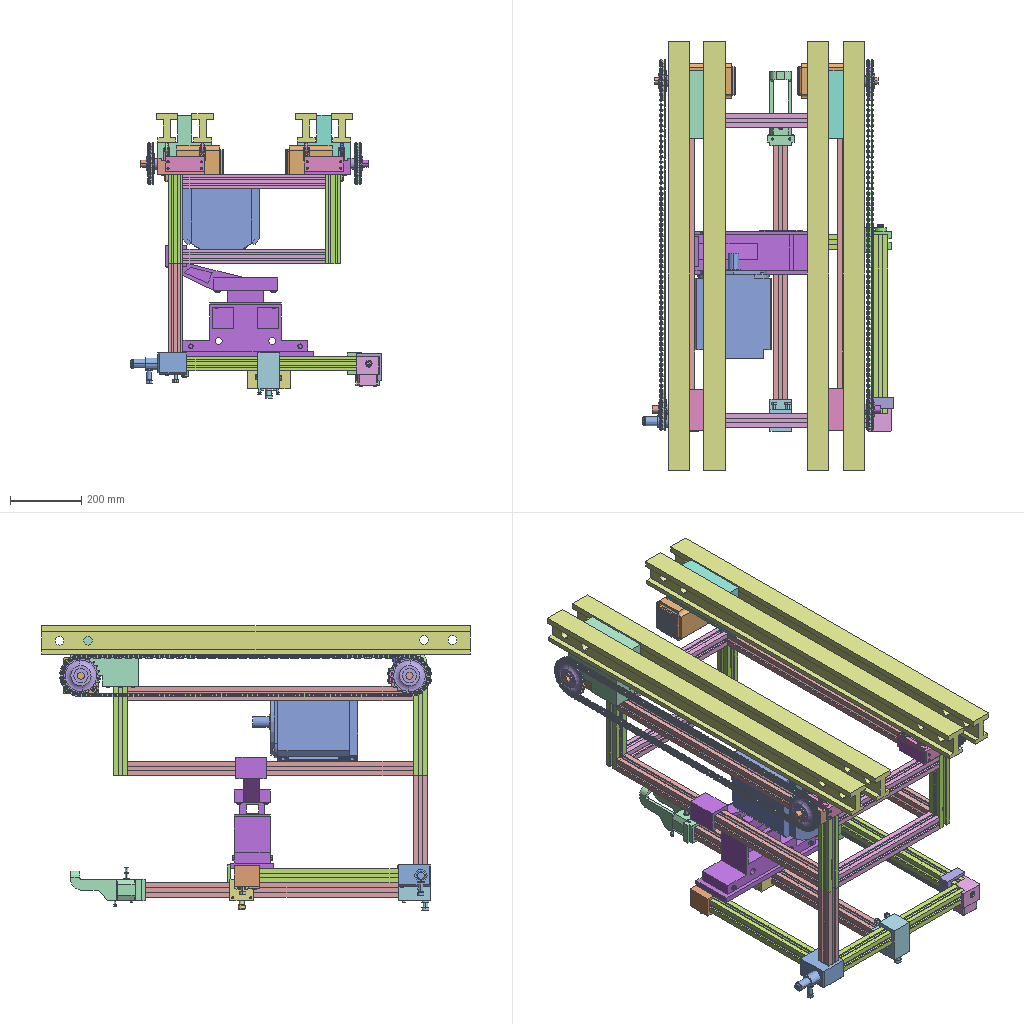Assembly | SolidWorks | 26 different items | 405 placed | box 701 x 1200 x 797 mm
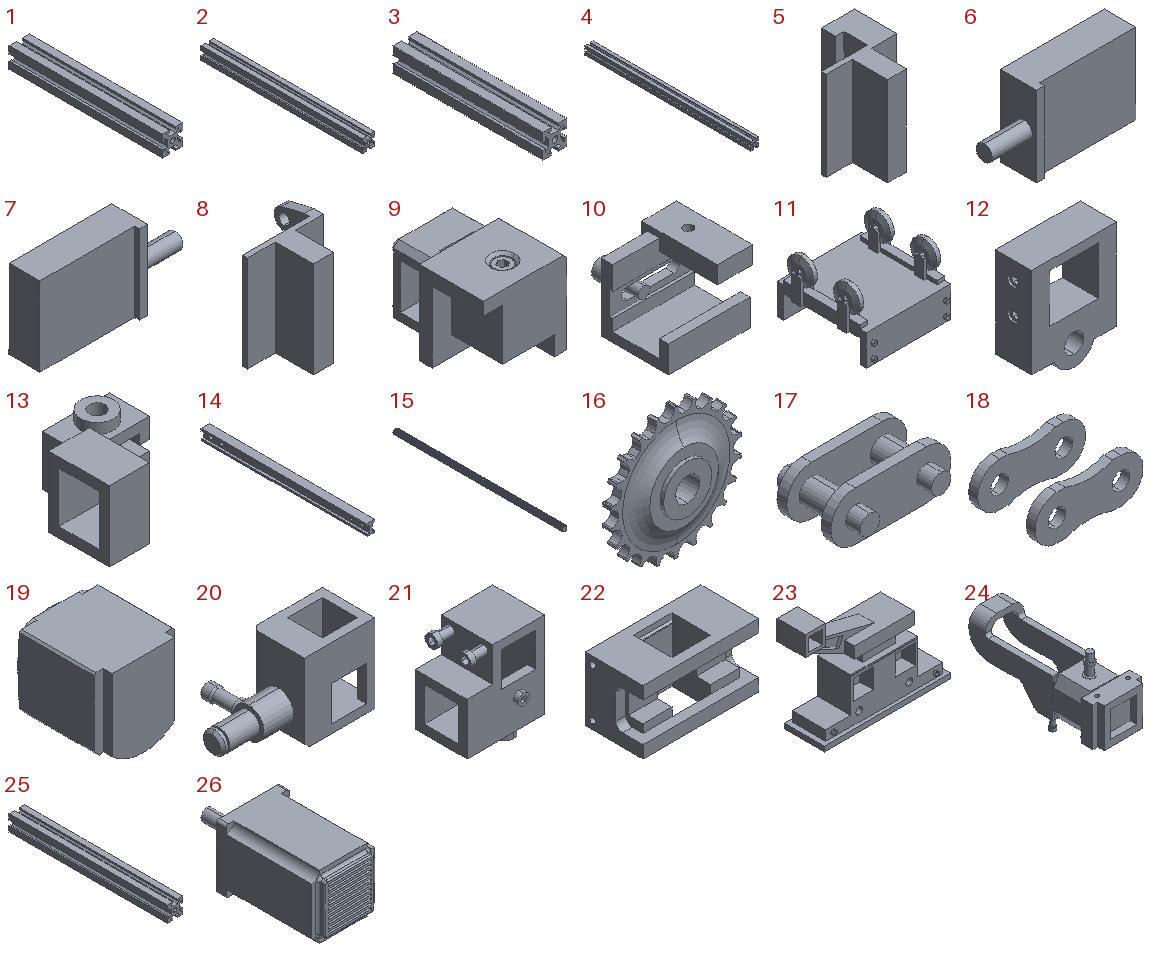Parts list (item | quantity | size | volume | features):
1 | x1 | 40 x 300 x 40 mm | 272732 mm3 | features Extrusion 1
2 | x4 | 40 x 500 x 40 mm | 454553 mm3 | features Extrusion 1
3 | x4 | 40 x 250 x 40 mm | 227277 mm3 | features Extrusion 1
4 | x5 | 40 x 800 x 40 mm | 727286 mm3 | features Extrusion 1
5 | x1 | 150 x 169 x 189.781 mm | 1407885 mm3 | features ICE 7, Extrusion 1, MirrorSolid 1
6 | x1 | 180 x 49 x 100 mm | 529109 mm3 | features ICE 6, Extrusion 1, MirrorSolid 1
7 | x1 | 180 x 49 x 100 mm | 529109 mm3 | features ICE 5, Extrusion 1
8 | x1 | 150 x 169 x 189.781 mm | 1407885 mm3 | features ICE 6, Extrusion 1
9 | x1 | 65 x 84 x 65 mm | 191550 mm3 | features ICE 10, Chamfer 3, Extrusion 1
10 | x1 | 70 x 83 x 63 mm | 98989 mm3 | features ICE 11, Extrusion 1
11 | x2 | 117 x 123 x 81 mm | 229130 mm3 | features ICE 7, LPattern 4, Chamfer 1, Extrusion 1, MirrorPattern 1, Revolution 1
12 | x1 | 70 x 30 x 86.838 mm | 111034 mm3 | features ICE 5, Extrusion 1, MirrorPattern 1
13 | x1 | 90 x 90 x 70 mm | 165265 mm3 | features ICE 5, Extrusion 1
14 | x4 | 60 x 1200 x 80 mm | 3164730 mm3 | features Extrusion 1, ICE 1
15 | x1 | 17 x 560 x 17 mm | 93030 mm3 | features Extrusion 1, Helix 1, ICE 1, Sweep 1
16 | x4 | 108.11 x 33 x 108.911 mm | 101426 mm3 | features ICE 2, Extrusion 1, RefAxis 1, RevCut 1
17 | x180 | 24.52 x 17 x 10 mm | 1321 mm3 | features ICE 4, RefPoint 2, Extrusion 1
18 | x180 | 24.52 x 15 x 10 mm | 736.592 mm3 | features ICE 2, Extrusion 1
19 | x1 | 215.394 x 294 x 225 mm | 10267409 mm3 | features ICE 13, Chamfer 1, CirPattern 1, Extrusion 1, MirrorPattern 1
20 | x1 | 156 x 86.375 x 90 mm | 325727 mm3 | features ICE 13, Chamfer 4, Extrusion 1
21 | x1 | 90 x 72 x 127 mm | 255195 mm3 | features ICE 12, Extrusion 1
22 | x1 | 120 x 84 x 66 mm | 274299 mm3 | features ICE 12, Chamfer 2, Fillet 2, Extrusion 1
23 | x1 | 415 x 120 x 311.384 mm | 4368887 mm3 | features ICE 14, MirrorPattern 9, Extrusion 1
24 | x1 | 75 x 208.792 x 108 mm | 304724 mm3 | features ICE 21, Fillet 6, MirrorPattern 3, Chamfer 2, Extrusion 1
25 | x4 | 40 x 400 x 40 mm | 363643 mm3 | features Extrusion 1
26 | x2 | 100 x 225 x 100 mm | 1510650 mm3 | features ICE 6, Fillet 3, CirPattern 1, Extrusion 1, LPattern 1
Mates (type | each side: item.copy, entity, surface, feature):
Coincident | 4.1 face plane Boss-Extrude1 | 3.1 face plane Boss-Extrude1 | 3 times
Coincident | 4.2 face plane Boss-Extrude1 | 3.2 face plane Boss-Extrude1 | 3 times
Coincident | 3.1 face plane Boss-Extrude1 | 25.1 face plane Boss-Extrude1 | 3 times
Coincident | 3.2 face plane Boss-Extrude1 | 25.1 face plane Boss-Extrude1 | 3 times
Coincident | 3.1 face plane Boss-Extrude1 | 25.2 face plane Boss-Extrude1
Coincident | 3.2 face plane Boss-Extrude1 | 25.2 face plane Boss-Extrude1 | 2 times
Coincident | 4.2 face plane Boss-Extrude1 | 3.3 face plane Boss-Extrude1 | 3 times
Coincident | 4.1 face plane Boss-Extrude1 | 3.4 face plane Boss-Extrude1 | 3 times
Coincident | 3.3 face plane Boss-Extrude1 | 25.3 face plane Boss-Extrude1 | 2 times
Coincident | 3.4 face plane Boss-Extrude1 | 25.3 face plane Boss-Extrude1
Coincident | 3.3 face plane Boss-Extrude1 | 25.4 face plane Boss-Extrude1 | 3 times
Coincident | 3.2 face plane Boss-Extrude1 | 4.3 face plane Boss-Extrude1 | 3 times
Coincident | 3.4 face plane Boss-Extrude1 | 4.4 face plane Boss-Extrude1 | 3 times
Coincident | 19.1 face plane Boss-Extrude2 | 4.4 face plane Boss-Extrude1
Coincident | 19.1 face plane Boss-Extrude5 | 4.4 face plane Boss-Extrude1
Concentric | 8.1 face cylinder Boss-Extrude4 | 26.1 face cylinder Boss-Extrude1
Coincident | 8.1 face plane Boss-Extrude4 | 26.1 face plane Boss-Extrude2
Concentric | 26.1 face cylinder Boss-Extrude1 | 16.1 face cylinder Boss-Extrude1
Coincident | 8.1 face plane Boss-Extrude1 | 16.1 face plane Boss-Extrude4
Coincident | 8.1 face plane Boss-Extrude7 | 14.1 face plane Boss-Extrude1
Coincident | 8.1 face plane Boss-Extrude6 | 14.1 face plane Boss-Extrude1
DistanceDim | 8.1 face plane Boss-Extrude5 | 14.1 face plane Boss-Extrude1
Coincident | 4.3 face plane Boss-Extrude1 | 7.1 face plane Boss-Extrude1
Coincident | 3.3 face plane Boss-Extrude1 | 7.1 face plane Boss-Extrude1
Concentric | 7.1 face cylinder Boss-Extrude3 | 16.2 face cylinder Boss-Extrude1
Coincident | 4.3 face plane Boss-Extrude1 | 8.1 face plane Boss-Extrude1 | 2 times
Coincident | 7.1 face plane Boss-Extrude1 | 16.2 face plane Boss-Extrude4
BeltDim | 16.1 face cylinder Cut-Revolve1 | 16.2 face cylinder Cut-Revolve1
Coincident | 8.1 face plane Boss-Extrude6 | 14.2 face plane Boss-Extrude1
Coincident | 8.1 face plane Boss-Extrude7 | 14.2 face plane Boss-Extrude1
Coincident | 14.1 face plane Boss-Extrude1 | 14.2 face plane Boss-Extrude1
DistanceDim | 25.2 face plane Boss-Extrude1 | 8.1 face plane Boss-Extrude1
Concentric | 26.2 face cylinder Boss-Extrude1 | 5.1 face cylinder Mirror3
Coincident | 14.3 face plane Boss-Extrude1 | 5.1 face plane Boss-Extrude7
Coincident | 4.4 face plane Boss-Extrude1 | 5.1 face plane Mirror3
Coincident | 3.4 face plane Boss-Extrude1 | 6.1 face plane Boss-Extrude1
Coincident | 4.4 face plane Boss-Extrude1 | 6.1 face plane Boss-Extrude1
Concentric | 6.1 face cylinder Mirror1 | 16.3 face cylinder Boss-Extrude1
Coincident | 6.1 face plane Mirror1 | 16.3 face plane Boss-Extrude4
Concentric | 26.2 face cylinder Boss-Extrude1 | 16.4 face cylinder Boss-Extrude1
Coincident | 5.1 face plane Boss-Extrude1 | 16.4 face plane Boss-Extrude4
Tangent | 14.1 face plane Boss-Extrude1 | 11.1 face cylinder LPattern4
DistanceDim | 11.1 face plane LPattern4 | 14.1 face plane Boss-Extrude1
Coincident | 7.1 face plane Boss-Extrude1 | 11.1 face plane Boss-Extrude1
Coincident | 8.1 face plane Boss-Extrude6 | 26.1 face plane Boss-Extrude3
Coincident | 3.4 face plane Boss-Extrude1 | 1.1 face plane Boss-Extrude1 | 3 times
Coincident | 1.1 face plane Boss-Extrude1 | 20.1 face plane Cut-Extrude1 | 3 times
Coincident | 1.1 face plane Boss-Extrude1 | 2.1 face plane Boss-Extrude1
Coincident | 20.1 face plane Cut-Extrude3 | 2.1 face plane Boss-Extrude1
Coincident | 20.1 face plane Cut-Extrude1 | 2.1 face plane Boss-Extrude1
Coincident | 20.1 face plane Cut-Extrude1 | 2.2 face plane Boss-Extrude1 | 2 times
Coincident | 1.1 face plane Boss-Extrude1 | 2.2 face plane Boss-Extrude1
Coincident | 2.2 face plane Boss-Extrude1 | 2.3 face plane Boss-Extrude1 | 3 times
Coincident | 2.3 face plane Boss-Extrude1 | 2.4 face plane Boss-Extrude1 | 2 times
Coincident | 2.3 face plane Boss-Extrude1 | 9.1 face plane Boss-Extrude1
Coincident | 2.2 face plane Boss-Extrude1 | 9.1 face plane Boss-Extrude1
Coincident | 2.2 face plane Boss-Extrude1 | 9.1 face plane Boss-Extrude3
Coincident | 2.1 face plane Boss-Extrude1 | 2.4 face plane Boss-Extrude1
Coincident | 2.1 face plane Boss-Extrude1 | 10.1 face plane Boss-Extrude1 | 2 times
Coincident | 2.3 face plane Boss-Extrude1 | 12.1 face plane Boss-Extrude1 | 2 times
Coincident | 9.1 face plane Boss-Extrude1 | 12.1 face plane Boss-Extrude1
Coincident | 2.1 face plane Boss-Extrude1 | 10.1 face plane Boss-Extrude8
Coincident | 2.4 face plane Boss-Extrude1 | 13.1 face plane Boss-Extrude3 | 2 times
Coincident | 2.3 face plane Boss-Extrude1 | 13.1 face plane Boss-Extrude3
Concentric | 13.1 face cylinder Cut-Extrude1 | 15.1 face cylinder Boss-Extrude1
DistanceDim | 13.1 face plane Boss-Extrude5 | 15.1 face plane Cut-Extrude1
Coincident | 2.2 face plane Boss-Extrude1 | 21.1 face plane Boss-Extrude1
Coincident | 2.2 face plane Boss-Extrude1 | 21.1 face plane Cut-Extrude2
DistanceDim | 21.1 face plane Boss-Extrude1 | 9.1 face plane Boss-Extrude1
Coincident | 21.1 face plane Cut-Extrude1 | 4.5 face plane Boss-Extrude1 | 2 times
Coincident | 21.1 face plane Boss-Extrude1 | 4.5 face plane Boss-Extrude1
Coincident | 2.4 face plane Boss-Extrude1 | 22.1 face plane Cut-Extrude1 | 2 times
Coincident | 4.5 face plane Boss-Extrude1 | 22.1 face plane Cut-Extrude2
Coincident | 2.4 face plane Boss-Extrude1 | 23.1 face plane Boss-Extrude1 | 3 times
Coincident | 4.5 face plane Boss-Extrude1 | 24.1 face plane Boss-Extrude1 | 2 times
Coincident | 4.5 face plane Boss-Extrude1 | 24.1 face plane Boss-Extrude2